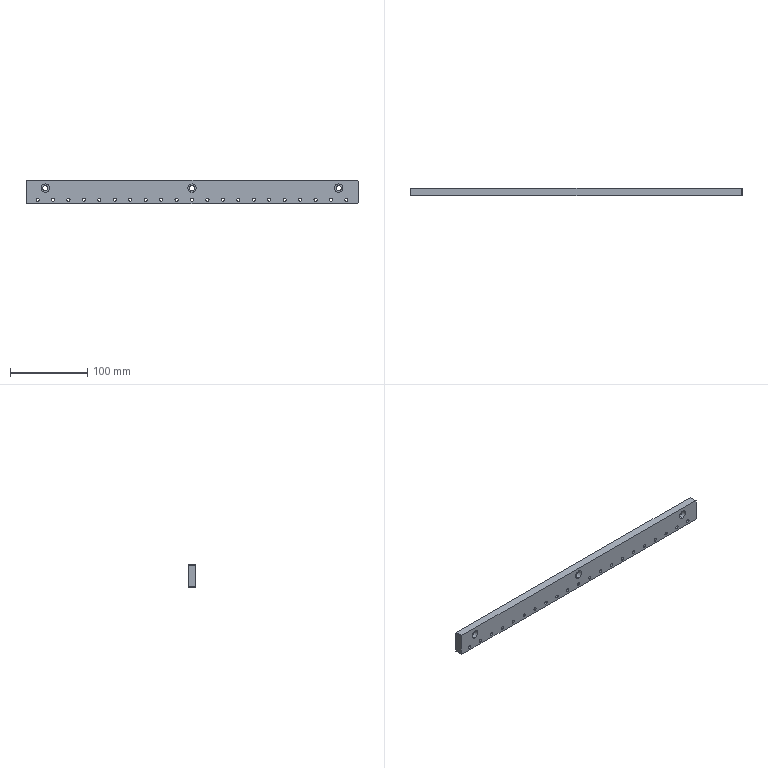Part | SolidWorks | features HoleWzd 2, Chamfer 1, Extrusion 1 | 1 solid | 67 faces | box 430 x 10 x 30 mm | volume 124086 mm3 | cylinder 54 | plane 13 | commonest cylinder face diameters 4.1 x42 6.6 x6 11 x6